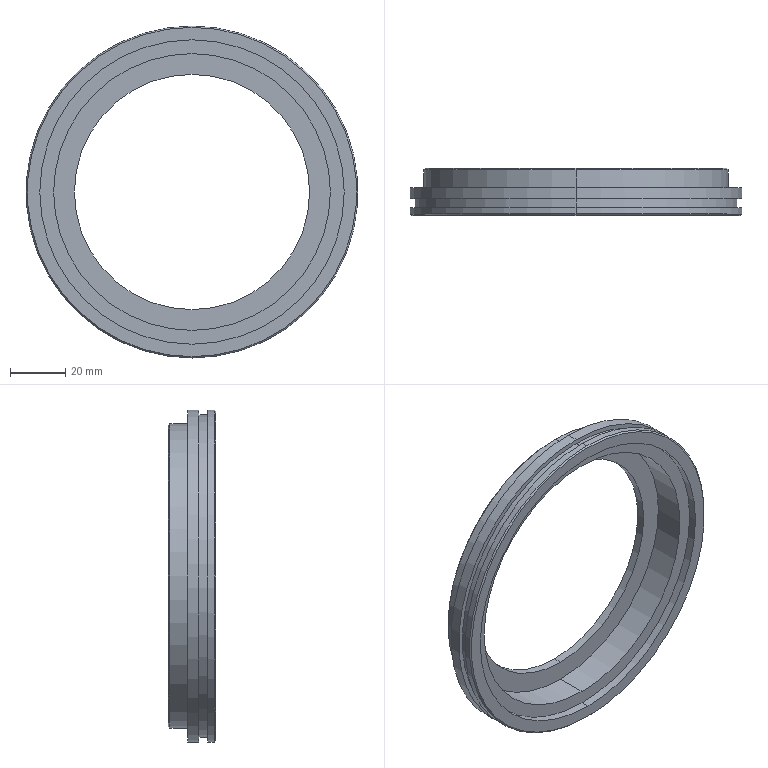Part | SolidWorks | features ICE 5, Chamfer 2, Extrusion 1 | 1 solid | 25 faces | box 120 x 17 x 120 mm | volume 45523 mm3 | cylinder 14 | plane 7 | cone 4 | commonest cylinder face diameters 110 x4 120 x4 85 x2 100 x2 116.5 x2
STEP:
#1=CARTESIAN_POINT('',(0.,17.,54.5));
#2=VERTEX_POINT('',#1);
#3=CARTESIAN_POINT('',(0.,17.,-54.5));
#4=VERTEX_POINT('',#3);
#5=CARTESIAN_POINT('',(0.,17.,0.));
#6=DIRECTION('',(0.,1.,0.));
#7=DIRECTION('',(0.,0.,1.));
#8=AXIS2_PLACEMENT_3D('',#5,#6,#7);
#9=CIRCLE('',#8,54.5);
#10=EDGE_CURVE('',#2,#4,#9,.T.);
#11=ORIENTED_EDGE('',*,*,#10,.F.);
#12=CARTESIAN_POINT('',(0.,16.5,55.));
#13=VERTEX_POINT('',#12);
#14=CARTESIAN_POINT('',(0.,17.,54.5));
#15=DIRECTION('',(0.,-0.7071,0.7071));
#16=VECTOR('',#15,1000.);
#17=LINE('',#14,#16);
#18=EDGE_CURVE('',#2,#13,#17,.T.);
#19=ORIENTED_EDGE('',*,*,#18,.T.);
#20=CARTESIAN_POINT('',(0.,16.5,-55.));
#21=VERTEX_POINT('',#20);
#22=CARTESIAN_POINT('',(0.,16.5,0.));
#23=DIRECTION('',(0.,-1.,0.));
#24=DIRECTION('',(0.,0.,1.));
#25=AXIS2_PLACEMENT_3D('',#22,#23,#24);
#26=CIRCLE('',#25,55.);
#27=EDGE_CURVE('',#21,#13,#26,.T.);
#28=ORIENTED_EDGE('',*,*,#27,.F.);
#29=CARTESIAN_POINT('',(0.,17.,-54.5));
#30=DIRECTION('',(0.,-0.7071,-0.7071));
#31=VECTOR('',#30,1000.);
#32=LINE('',#29,#31);
#33=EDGE_CURVE('',#4,#21,#32,.T.);
#34=ORIENTED_EDGE('',*,*,#33,.F.);
#35=EDGE_LOOP('',(#11,#19,#28,#34));
#36=FACE_OUTER_BOUND('',#35,.T.);
#37=CARTESIAN_POINT('',(0.,17.,0.));
#38=DIRECTION('',(0.,-1.,0.));
#39=DIRECTION('',(0.,0.,-1.));
#40=AXIS2_PLACEMENT_3D('',#37,#38,#39);
#41=CONICAL_SURFACE('',#40,54.5,0.7854);
#42=ADVANCED_FACE('',(#36),#41,.T.);
#43=CARTESIAN_POINT('',(0.,0.,-59.5));
#44=VERTEX_POINT('',#43);
#45=CARTESIAN_POINT('',(0.,0.,59.5));
#46=VERTEX_POINT('',#45);
#47=CARTESIAN_POINT('',(0.,0.,0.));
#48=DIRECTION('',(0.,-1.,0.));
#49=DIRECTION('',(0.,0.,1.));
#50=AXIS2_PLACEMENT_3D('',#47,#48,#49);
#51=CIRCLE('',#50,59.5);
#52=EDGE_CURVE('',#44,#46,#51,.T.);
#53=ORIENTED_EDGE('',*,*,#52,.F.);
#54=CARTESIAN_POINT('',(0.,0.5,-60.));
#55=VERTEX_POINT('',#54);
#56=CARTESIAN_POINT('',(0.,0.5,-60.));
#57=DIRECTION('',(0.,0.7071,-0.7071));
#58=VECTOR('',#57,1000.);
#59=LINE('',#56,#58);
#60=EDGE_CURVE('',#44,#55,#59,.T.);
#61=ORIENTED_EDGE('',*,*,#60,.T.);
#62=CARTESIAN_POINT('',(0.,0.5,60.));
#63=VERTEX_POINT('',#62);
#64=CARTESIAN_POINT('',(0.,0.5,0.));
#65=DIRECTION('',(0.,1.,0.));
#66=DIRECTION('',(0.,0.,1.));
#67=AXIS2_PLACEMENT_3D('',#64,#65,#66);
#68=CIRCLE('',#67,60.);
#69=EDGE_CURVE('',#63,#55,#68,.T.);
#70=ORIENTED_EDGE('',*,*,#69,.F.);
#71=CARTESIAN_POINT('',(0.,0.5,60.));
#72=DIRECTION('',(0.,0.7071,0.7071));
#73=VECTOR('',#72,1000.);
#74=LINE('',#71,#73);
#75=EDGE_CURVE('',#46,#63,#74,.T.);
#76=ORIENTED_EDGE('',*,*,#75,.F.);
#77=EDGE_LOOP('',(#53,#61,#70,#76));
#78=FACE_OUTER_BOUND('',#77,.T.);
#79=CARTESIAN_POINT('',(0.,0.5,0.));
#80=DIRECTION('',(0.,1.,0.));
#81=DIRECTION('',(0.,0.,1.));
#82=AXIS2_PLACEMENT_3D('',#79,#80,#81);
#83=CONICAL_SURFACE('',#82,60.,0.7854);
#84=ADVANCED_FACE('',(#78),#83,.T.);
#85=CARTESIAN_POINT('',(0.,2.8,-58.25));
#86=VERTEX_POINT('',#85);
#87=CARTESIAN_POINT('',(0.,2.8,58.25));
#88=VERTEX_POINT('',#87);
#89=CARTESIAN_POINT('',(0.,2.8,0.));
#90=DIRECTION('',(0.,-1.,0.));
#91=DIRECTION('',(0.,0.,-1.));
#92=AXIS2_PLACEMENT_3D('',#89,#90,#91);
#93=CIRCLE('',#92,58.25);
#94=EDGE_CURVE('',#86,#88,#93,.T.);
#95=ORIENTED_EDGE('',*,*,#94,.F.);
#96=CARTESIAN_POINT('',(0.,6.,-58.25));
#97=VERTEX_POINT('',#96);
#98=CARTESIAN_POINT('',(0.,2.8,-58.25));
#99=DIRECTION('',(0.,1.,0.));
#100=VECTOR('',#99,1000.);
#101=LINE('',#98,#100);
#102=EDGE_CURVE('',#86,#97,#101,.T.);
#103=ORIENTED_EDGE('',*,*,#102,.T.);
#104=CARTESIAN_POINT('',(0.,6.,58.25));
#105=VERTEX_POINT('',#104);
#106=CARTESIAN_POINT('',(0.,6.,0.));
#107=DIRECTION('',(0.,-1.,0.));
#108=DIRECTION('',(0.,0.,-1.));
#109=AXIS2_PLACEMENT_3D('',#106,#107,#108);
#110=CIRCLE('',#109,58.25);
#111=EDGE_CURVE('',#97,#105,#110,.T.);
#112=ORIENTED_EDGE('',*,*,#111,.T.);
#113=CARTESIAN_POINT('',(0.,2.8,58.25));
#114=DIRECTION('',(0.,1.,0.));
#115=VECTOR('',#114,1000.);
#116=LINE('',#113,#115);
#117=EDGE_CURVE('',#88,#105,#116,.T.);
#118=ORIENTED_EDGE('',*,*,#117,.F.);
#119=EDGE_LOOP('',(#95,#103,#112,#118));
#120=FACE_OUTER_BOUND('',#119,.T.);
#121=CARTESIAN_POINT('',(0.,2.8,0.));
#122=DIRECTION('',(0.,1.,0.));
#123=DIRECTION('',(0.,0.,1.));
#124=AXIS2_PLACEMENT_3D('',#121,#122,#123);
#125=CYLINDRICAL_SURFACE('',#124,58.25);
#126=ADVANCED_FACE('',(#120),#125,.T.);
#127=CARTESIAN_POINT('',(0.,14.,50.));
#128=VERTEX_POINT('',#127);
#129=CARTESIAN_POINT('',(0.,14.,-50.));
#130=VERTEX_POINT('',#129);
#131=CARTESIAN_POINT('',(0.,14.,0.));
#132=DIRECTION('',(0.,-1.,0.));
#133=DIRECTION('',(0.,0.,-1.));
#134=AXIS2_PLACEMENT_3D('',#131,#132,#133);
#135=CIRCLE('',#134,50.);
#136=EDGE_CURVE('',#128,#130,#135,.T.);
#137=ORIENTED_EDGE('',*,*,#136,.F.);
#138=CARTESIAN_POINT('',(0.,3.,50.));
#139=VERTEX_POINT('',#138);
#140=CARTESIAN_POINT('',(0.,14.,50.));
#141=DIRECTION('',(0.,-1.,0.));
#142=VECTOR('',#141,1000.);
#143=LINE('',#140,#142);
#144=EDGE_CURVE('',#128,#139,#143,.T.);
#145=ORIENTED_EDGE('',*,*,#144,.T.);
#146=CARTESIAN_POINT('',(0.,3.,-50.));
#147=VERTEX_POINT('',#146);
#148=CARTESIAN_POINT('',(0.,3.,0.));
#149=DIRECTION('',(0.,-1.,0.));
#150=DIRECTION('',(0.,0.,-1.));
#151=AXIS2_PLACEMENT_3D('',#148,#149,#150);
#152=CIRCLE('',#151,50.);
#153=EDGE_CURVE('',#139,#147,#152,.T.);
#154=ORIENTED_EDGE('',*,*,#153,.T.);
#155=CARTESIAN_POINT('',(0.,14.,-50.));
#156=DIRECTION('',(0.,-1.,0.));
#157=VECTOR('',#156,1000.);
#158=LINE('',#155,#157);
#159=EDGE_CURVE('',#130,#147,#158,.T.);
#160=ORIENTED_EDGE('',*,*,#159,.F.);
#161=EDGE_LOOP('',(#137,#145,#154,#160));
#162=FACE_OUTER_BOUND('',#161,.T.);
#163=CARTESIAN_POINT('',(0.,14.,0.));
#164=DIRECTION('',(0.,-1.,0.));
#165=DIRECTION('',(0.,0.,-1.));
#166=AXIS2_PLACEMENT_3D('',#163,#164,#165);
#167=CYLINDRICAL_SURFACE('',#166,50.);
#168=ADVANCED_FACE('',(#162),#167,.F.);
#169=CARTESIAN_POINT('',(0.,3.,55.));
#170=VERTEX_POINT('',#169);
#171=CARTESIAN_POINT('',(0.,3.,-55.));
#172=VERTEX_POINT('',#171);
#173=CARTESIAN_POINT('',(0.,3.,0.));
#174=DIRECTION('',(0.,-1.,0.));
#175=DIRECTION('',(0.,0.,-1.));
#176=AXIS2_PLACEMENT_3D('',#173,#174,#175);
#177=CIRCLE('',#176,55.);
#178=EDGE_CURVE('',#170,#172,#177,.T.);
#179=ORIENTED_EDGE('',*,*,#178,.F.);
#180=CARTESIAN_POINT('',(0.,0.,55.));
#181=VERTEX_POINT('',#180);
#182=CARTESIAN_POINT('',(0.,3.,55.));
#183=DIRECTION('',(0.,-1.,0.));
#184=VECTOR('',#183,1000.);
#185=LINE('',#182,#184);
#186=EDGE_CURVE('',#170,#181,#185,.T.);
#187=ORIENTED_EDGE('',*,*,#186,.T.);
#188=CARTESIAN_POINT('',(0.,0.,-55.));
#189=VERTEX_POINT('',#188);
#190=CARTESIAN_POINT('',(0.,0.,0.));
#191=DIRECTION('',(0.,-1.,0.));
#192=DIRECTION('',(0.,0.,-1.));
#193=AXIS2_PLACEMENT_3D('',#190,#191,#192);
#194=CIRCLE('',#193,55.);
#195=EDGE_CURVE('',#181,#189,#194,.T.);
#196=ORIENTED_EDGE('',*,*,#195,.T.);
#197=CARTESIAN_POINT('',(0.,3.,-55.));
#198=DIRECTION('',(0.,-1.,0.));
#199=VECTOR('',#198,1000.);
#200=LINE('',#197,#199);
#201=EDGE_CURVE('',#172,#189,#200,.T.);
#202=ORIENTED_EDGE('',*,*,#201,.F.);
#203=EDGE_LOOP('',(#179,#187,#196,#202));
#204=FACE_OUTER_BOUND('',#203,.T.);
#205=CARTESIAN_POINT('',(0.,3.,0.));
#206=DIRECTION('',(0.,-1.,0.));
#207=DIRECTION('',(0.,0.,-1.));
#208=AXIS2_PLACEMENT_3D('',#205,#206,#207);
#209=CYLINDRICAL_SURFACE('',#208,55.);
#210=ADVANCED_FACE('',(#204),#209,.F.);
#211=ORIENTED_EDGE('',*,*,#27,.T.);
#212=CARTESIAN_POINT('',(0.,10.,55.));
#213=VERTEX_POINT('',#212);
#214=CARTESIAN_POINT('',(0.,17.,55.));
#215=DIRECTION('',(0.,-1.,0.));
#216=VECTOR('',#215,1000.);
#217=LINE('',#214,#216);
#218=EDGE_CURVE('',#13,#213,#217,.T.);
#219=ORIENTED_EDGE('',*,*,#218,.T.);
#220=CARTESIAN_POINT('',(0.,10.,-55.));
#221=VERTEX_POINT('',#220);
#222=CARTESIAN_POINT('',(0.,10.,0.));
#223=DIRECTION('',(0.,1.,0.));
#224=DIRECTION('',(0.,0.,1.));
#225=AXIS2_PLACEMENT_3D('',#222,#223,#224);
#226=CIRCLE('',#225,55.);
#227=EDGE_CURVE('',#213,#221,#226,.T.);
#228=ORIENTED_EDGE('',*,*,#227,.T.);
#229=CARTESIAN_POINT('',(0.,17.,-55.));
#230=DIRECTION('',(0.,-1.,0.));
#231=VECTOR('',#230,1000.);
#232=LINE('',#229,#231);
#233=EDGE_CURVE('',#21,#221,#232,.T.);
#234=ORIENTED_EDGE('',*,*,#233,.F.);
#235=EDGE_LOOP('',(#211,#219,#228,#234));
#236=FACE_OUTER_BOUND('',#235,.T.);
#237=CARTESIAN_POINT('',(0.,17.,0.));
#238=DIRECTION('',(0.,-1.,0.));
#239=DIRECTION('',(0.,0.,-1.));
#240=AXIS2_PLACEMENT_3D('',#237,#238,#239);
#241=CYLINDRICAL_SURFACE('',#240,55.);
#242=ADVANCED_FACE('',(#236),#241,.T.);
#243=CARTESIAN_POINT('',(0.,2.8,-60.));
#244=VERTEX_POINT('',#243);
#245=CARTESIAN_POINT('',(0.,2.8,60.));
#246=VERTEX_POINT('',#245);
#247=CARTESIAN_POINT('',(0.,2.8,0.));
#248=DIRECTION('',(0.,-1.,0.));
#249=DIRECTION('',(0.,0.,-1.));
#250=AXIS2_PLACEMENT_3D('',#247,#248,#249);
#251=CIRCLE('',#250,60.);
#252=EDGE_CURVE('',#244,#246,#251,.T.);
#253=ORIENTED_EDGE('',*,*,#252,.T.);
#254=CARTESIAN_POINT('',(0.,10.,60.));
#255=DIRECTION('',(0.,-1.,0.));
#256=VECTOR('',#255,1000.);
#257=LINE('',#254,#256);
#258=EDGE_CURVE('',#246,#63,#257,.T.);
#259=ORIENTED_EDGE('',*,*,#258,.T.);
#260=ORIENTED_EDGE('',*,*,#69,.T.);
#261=CARTESIAN_POINT('',(0.,10.,-60.));
#262=DIRECTION('',(0.,-1.,0.));
#263=VECTOR('',#262,1000.);
#264=LINE('',#261,#263);
#265=EDGE_CURVE('',#244,#55,#264,.T.);
#266=ORIENTED_EDGE('',*,*,#265,.F.);
#267=EDGE_LOOP('',(#253,#259,#260,#266));
#268=FACE_OUTER_BOUND('',#267,.T.);
#269=CARTESIAN_POINT('',(0.,10.,0.));
#270=DIRECTION('',(0.,-1.,0.));
#271=DIRECTION('',(0.,0.,-1.));
#272=AXIS2_PLACEMENT_3D('',#269,#270,#271);
#273=CYLINDRICAL_SURFACE('',#272,60.);
#274=ADVANCED_FACE('',(#268),#273,.T.);
#275=CARTESIAN_POINT('',(0.,14.,-42.5));
#276=VERTEX_POINT('',#275);
#277=CARTESIAN_POINT('',(0.,14.,42.5));
#278=VERTEX_POINT('',#277);
#279=CARTESIAN_POINT('',(0.,14.,0.));
#280=DIRECTION('',(0.,1.,0.));
#281=DIRECTION('',(0.,0.,-1.));
#282=AXIS2_PLACEMENT_3D('',#279,#280,#281);
#283=CIRCLE('',#282,42.5);
#284=EDGE_CURVE('',#276,#278,#283,.T.);
#285=ORIENTED_EDGE('',*,*,#284,.F.);
#286=CARTESIAN_POINT('',(0.,17.,-42.5));
#287=VERTEX_POINT('',#286);
#288=CARTESIAN_POINT('',(0.,0.,-42.5));
#289=DIRECTION('',(0.,1.,0.));
#290=VECTOR('',#289,1000.);
#291=LINE('',#288,#290);
#292=EDGE_CURVE('',#276,#287,#291,.T.);
#293=ORIENTED_EDGE('',*,*,#292,.T.);
#294=CARTESIAN_POINT('',(0.,17.,42.5));
#295=VERTEX_POINT('',#294);
#296=CARTESIAN_POINT('',(0.,17.,0.));
#297=DIRECTION('',(0.,1.,0.));
#298=DIRECTION('',(0.,0.,1.));
#299=AXIS2_PLACEMENT_3D('',#296,#297,#298);
#300=CIRCLE('',#299,42.5);
#301=EDGE_CURVE('',#287,#295,#300,.T.);
#302=ORIENTED_EDGE('',*,*,#301,.T.);
#303=CARTESIAN_POINT('',(0.,0.,42.5));
#304=DIRECTION('',(0.,1.,0.));
#305=VECTOR('',#304,1000.);
#306=LINE('',#303,#305);
#307=EDGE_CURVE('',#278,#295,#306,.T.);
#308=ORIENTED_EDGE('',*,*,#307,.F.);
#309=EDGE_LOOP('',(#285,#293,#302,#308));
#310=FACE_OUTER_BOUND('',#309,.T.);
#311=CARTESIAN_POINT('',(0.,0.,0.));
#312=DIRECTION('',(0.,1.,0.));
#313=DIRECTION('',(0.,0.,1.));
#314=AXIS2_PLACEMENT_3D('',#311,#312,#313);
#315=CYLINDRICAL_SURFACE('',#314,42.5);
#316=ADVANCED_FACE('',(#310),#315,.F.);
#317=CARTESIAN_POINT('',(0.,10.,60.));
#318=VERTEX_POINT('',#317);
#319=CARTESIAN_POINT('',(0.,10.,-60.));
#320=VERTEX_POINT('',#319);
#321=CARTESIAN_POINT('',(0.,10.,0.));
#322=DIRECTION('',(0.,1.,0.));
#323=DIRECTION('',(0.,0.,1.));
#324=AXIS2_PLACEMENT_3D('',#321,#322,#323);
#325=CIRCLE('',#324,60.);
#326=EDGE_CURVE('',#318,#320,#325,.T.);
#327=ORIENTED_EDGE('',*,*,#326,.F.);
#328=CARTESIAN_POINT('',(0.,6.,60.));
#329=VERTEX_POINT('',#328);
#330=CARTESIAN_POINT('',(0.,10.,60.));
#331=DIRECTION('',(0.,-1.,0.));
#332=VECTOR('',#331,1000.);
#333=LINE('',#330,#332);
#334=EDGE_CURVE('',#318,#329,#333,.T.);
#335=ORIENTED_EDGE('',*,*,#334,.T.);
#336=CARTESIAN_POINT('',(0.,6.,-60.));
#337=VERTEX_POINT('',#336);
#338=CARTESIAN_POINT('',(0.,6.,0.));
#339=DIRECTION('',(0.,-1.,0.));
#340=DIRECTION('',(0.,0.,-1.));
#341=AXIS2_PLACEMENT_3D('',#338,#339,#340);
#342=CIRCLE('',#341,60.);
#343=EDGE_CURVE('',#337,#329,#342,.T.);
#344=ORIENTED_EDGE('',*,*,#343,.F.);
#345=CARTESIAN_POINT('',(0.,10.,-60.));
#346=DIRECTION('',(0.,-1.,0.));
#347=VECTOR('',#346,1000.);
#348=LINE('',#345,#347);
#349=EDGE_CURVE('',#320,#337,#348,.T.);
#350=ORIENTED_EDGE('',*,*,#349,.F.);
#351=EDGE_LOOP('',(#327,#335,#344,#350));
#352=FACE_OUTER_BOUND('',#351,.T.);
#353=CARTESIAN_POINT('',(0.,10.,0.));
#354=DIRECTION('',(0.,-1.,0.));
#355=DIRECTION('',(0.,0.,-1.));
#356=AXIS2_PLACEMENT_3D('',#353,#354,#355);
#357=CYLINDRICAL_SURFACE('',#356,60.);
#358=ADVANCED_FACE('',(#352),#357,.T.);
#359=ORIENTED_EDGE('',*,*,#334,.F.);
#360=CARTESIAN_POINT('',(0.,10.,0.));
#361=DIRECTION('',(0.,1.,0.));
#362=DIRECTION('',(0.,0.,1.));
#363=AXIS2_PLACEMENT_3D('',#360,#361,#362);
#364=CIRCLE('',#363,60.);
#365=EDGE_CURVE('',#320,#318,#364,.T.);
#366=ORIENTED_EDGE('',*,*,#365,.F.);
#367=ORIENTED_EDGE('',*,*,#349,.T.);
#368=CARTESIAN_POINT('',(0.,6.,0.));
#369=DIRECTION('',(0.,-1.,0.));
#370=DIRECTION('',(0.,0.,-1.));
#371=AXIS2_PLACEMENT_3D('',#368,#369,#370);
#372=CIRCLE('',#371,60.);
#373=EDGE_CURVE('',#329,#337,#372,.T.);
#374=ORIENTED_EDGE('',*,*,#373,.F.);
#375=EDGE_LOOP('',(#359,#366,#367,#374));
#376=FACE_OUTER_BOUND('',#375,.T.);
#377=CARTESIAN_POINT('',(0.,10.,0.));
#378=DIRECTION('',(0.,-1.,0.));
#379=DIRECTION('',(0.,0.,-1.));
#380=AXIS2_PLACEMENT_3D('',#377,#378,#379);
#381=CYLINDRICAL_SURFACE('',#380,60.);
#382=ADVANCED_FACE('',(#376),#381,.T.);
#383=ORIENTED_EDGE('',*,*,#292,.F.);
#384=CARTESIAN_POINT('',(0.,14.,0.));
#385=DIRECTION('',(0.,1.,0.));
#386=DIRECTION('',(0.,0.,-1.));
#387=AXIS2_PLACEMENT_3D('',#384,#385,#386);
#388=CIRCLE('',#387,42.5);
#389=EDGE_CURVE('',#278,#276,#388,.T.);
#390=ORIENTED_EDGE('',*,*,#389,.F.);
#391=ORIENTED_EDGE('',*,*,#307,.T.);
#392=CARTESIAN_POINT('',(0.,17.,0.));
#393=DIRECTION('',(0.,1.,0.));
#394=DIRECTION('',(0.,0.,1.));
#395=AXIS2_PLACEMENT_3D('',#392,#393,#394);
#396=CIRCLE('',#395,42.5);
#397=EDGE_CURVE('',#295,#287,#396,.T.);
#398=ORIENTED_EDGE('',*,*,#397,.T.);
#399=EDGE_LOOP('',(#383,#390,#391,#398));
#400=FACE_OUTER_BOUND('',#399,.T.);
#401=CARTESIAN_POINT('',(0.,0.,0.));
#402=DIRECTION('',(0.,1.,0.));
#403=DIRECTION('',(0.,0.,1.));
#404=AXIS2_PLACEMENT_3D('',#401,#402,#403);
#405=CYLINDRICAL_SURFACE('',#404,42.5);
#406=ADVANCED_FACE('',(#400),#405,.F.);
#407=ORIENTED_EDGE('',*,*,#258,.F.);
#408=CARTESIAN_POINT('',(0.,2.8,0.));
#409=DIRECTION('',(0.,-1.,0.));
#410=DIRECTION('',(0.,0.,-1.));
#411=AXIS2_PLACEMENT_3D('',#408,#409,#410);
#412=CIRCLE('',#411,60.);
#413=EDGE_CURVE('',#246,#244,#412,.T.);
#414=ORIENTED_EDGE('',*,*,#413,.T.);
#415=ORIENTED_EDGE('',*,*,#265,.T.);
#416=CARTESIAN_POINT('',(0.,0.5,0.));
#417=DIRECTION('',(0.,1.,0.));
#418=DIRECTION('',(0.,0.,1.));
#419=AXIS2_PLACEMENT_3D('',#416,#417,#418);
#420=CIRCLE('',#419,60.);
#421=EDGE_CURVE('',#55,#63,#420,.T.);
#422=ORIENTED_EDGE('',*,*,#421,.T.);
#423=EDGE_LOOP('',(#407,#414,#415,#422));
#424=FACE_OUTER_BOUND('',#423,.T.);
#425=CARTESIAN_POINT('',(0.,10.,0.));
#426=DIRECTION('',(0.,-1.,0.));
#427=DIRECTION('',(0.,0.,-1.));
#428=AXIS2_PLACEMENT_3D('',#425,#426,#427);
#429=CYLINDRICAL_SURFACE('',#428,60.);
#430=ADVANCED_FACE('',(#424),#429,.T.);
#431=CARTESIAN_POINT('',(0.,10.,0.));
#432=DIRECTION('',(0.,1.,0.));
#433=DIRECTION('',(0.,0.,1.));
#434=AXIS2_PLACEMENT_3D('',#431,#432,#433);
#435=CIRCLE('',#434,55.);
#436=EDGE_CURVE('',#221,#213,#435,.T.);
#437=ORIENTED_EDGE('',*,*,#436,.F.);
#438=ORIENTED_EDGE('',*,*,#227,.F.);
#439=EDGE_LOOP('',(#437,#438));
#440=FACE_BOUND('',#439,.T.);
#441=ORIENTED_EDGE('',*,*,#365,.T.);
#442=ORIENTED_EDGE('',*,*,#326,.T.);
#443=EDGE_LOOP('',(#441,#442));
#444=FACE_OUTER_BOUND('',#443,.T.);
#445=CARTESIAN_POINT('',(0.,10.,0.));
#446=DIRECTION('',(0.,1.,0.));
#447=DIRECTION('',(0.,0.,1.));
#448=AXIS2_PLACEMENT_3D('',#445,#446,#447);
#449=PLANE('',#448);
#450=ADVANCED_FACE('',(#440,#444),#449,.T.);
#451=CARTESIAN_POINT('',(0.,0.,0.));
#452=DIRECTION('',(0.,-1.,0.));
#453=DIRECTION('',(0.,0.,1.));
#454=AXIS2_PLACEMENT_3D('',#451,#452,#453);
#455=CIRCLE('',#454,59.5);
#456=EDGE_CURVE('',#46,#44,#455,.T.);
#457=ORIENTED_EDGE('',*,*,#456,.T.);
#458=ORIENTED_EDGE('',*,*,#52,.T.);
#459=EDGE_LOOP('',(#457,#458));
#460=FACE_OUTER_BOUND('',#459,.T.);
#461=CARTESIAN_POINT('',(0.,0.,0.));
#462=DIRECTION('',(0.,-1.,0.));
#463=DIRECTION('',(0.,0.,-1.));
#464=AXIS2_PLACEMENT_3D('',#461,#462,#463);
#465=CIRCLE('',#464,55.);
#466=EDGE_CURVE('',#189,#181,#465,.T.);
#467=ORIENTED_EDGE('',*,*,#466,.F.);
#468=ORIENTED_EDGE('',*,*,#195,.F.);
#469=EDGE_LOOP('',(#467,#468));
#470=FACE_BOUND('',#469,.T.);
#471=CARTESIAN_POINT('',(0.,0.,0.));
#472=DIRECTION('',(0.,1.,0.));
#473=DIRECTION('',(0.,0.,1.));
#474=AXIS2_PLACEMENT_3D('',#471,#472,#473);
#475=PLANE('',#474);
#476=ADVANCED_FACE('',(#460,#470),#475,.F.);
#477=ORIENTED_EDGE('',*,*,#218,.F.);
#478=CARTESIAN_POINT('',(0.,16.5,0.));
#479=DIRECTION('',(0.,-1.,0.));
#480=DIRECTION('',(0.,0.,1.));
#481=AXIS2_PLACEMENT_3D('',#478,#479,#480);
#482=CIRCLE('',#481,55.);
#483=EDGE_CURVE('',#13,#21,#482,.T.);
#484=ORIENTED_EDGE('',*,*,#483,.T.);
#485=ORIENTED_EDGE('',*,*,#233,.T.);
#486=ORIENTED_EDGE('',*,*,#436,.T.);
#487=EDGE_LOOP('',(#477,#484,#485,#486));
#488=FACE_OUTER_BOUND('',#487,.T.);
#489=CARTESIAN_POINT('',(0.,17.,0.));
#490=DIRECTION('',(0.,-1.,0.));
#491=DIRECTION('',(0.,0.,-1.));
#492=AXIS2_PLACEMENT_3D('',#489,#490,#491);
#493=CYLINDRICAL_SURFACE('',#492,55.);
#494=ADVANCED_FACE('',(#488),#493,.T.);
#495=CARTESIAN_POINT('',(0.,17.,0.));
#496=DIRECTION('',(0.,1.,0.));
#497=DIRECTION('',(0.,0.,1.));
#498=AXIS2_PLACEMENT_3D('',#495,#496,#497);
#499=CIRCLE('',#498,54.5);
#500=EDGE_CURVE('',#4,#2,#499,.T.);
#501=ORIENTED_EDGE('',*,*,#500,.T.);
#502=ORIENTED_EDGE('',*,*,#10,.T.);
#503=EDGE_LOOP('',(#501,#502));
#504=FACE_OUTER_BOUND('',#503,.T.);
#505=ORIENTED_EDGE('',*,*,#397,.F.);
#506=ORIENTED_EDGE('',*,*,#301,.F.);
#507=EDGE_LOOP('',(#505,#506));
#508=FACE_BOUND('',#507,.T.);
#509=CARTESIAN_POINT('',(0.,17.,0.));
#510=DIRECTION('',(0.,1.,0.));
#511=DIRECTION('',(0.,0.,1.));
#512=AXIS2_PLACEMENT_3D('',#509,#510,#511);
#513=PLANE('',#512);
#514=ADVANCED_FACE('',(#504,#508),#513,.T.);
#515=CARTESIAN_POINT('',(0.,3.,0.));
#516=DIRECTION('',(0.,-1.,0.));
#517=DIRECTION('',(0.,0.,-1.));
#518=AXIS2_PLACEMENT_3D('',#515,#516,#517);
#519=CIRCLE('',#518,50.);
#520=EDGE_CURVE('',#147,#139,#519,.T.);
#521=ORIENTED_EDGE('',*,*,#520,.F.);
#522=ORIENTED_EDGE('',*,*,#153,.F.);
#523=EDGE_LOOP('',(#521,#522));
#524=FACE_BOUND('',#523,.T.);
#525=CARTESIAN_POINT('',(0.,3.,0.));
#526=DIRECTION('',(0.,-1.,0.));
#527=DIRECTION('',(0.,0.,-1.));
#528=AXIS2_PLACEMENT_3D('',#525,#526,#527);
#529=CIRCLE('',#528,55.);
#530=EDGE_CURVE('',#172,#170,#529,.T.);
#531=ORIENTED_EDGE('',*,*,#530,.T.);
#532=ORIENTED_EDGE('',*,*,#178,.T.);
#533=EDGE_LOOP('',(#531,#532));
#534=FACE_OUTER_BOUND('',#533,.T.);
#535=CARTESIAN_POINT('',(0.,3.,0.));
#536=DIRECTION('',(0.,-1.,0.));
#537=DIRECTION('',(0.,0.,-1.));
#538=AXIS2_PLACEMENT_3D('',#535,#536,#537);
#539=PLANE('',#538);
#540=ADVANCED_FACE('',(#524,#534),#539,.T.);
#541=ORIENTED_EDGE('',*,*,#186,.F.);
#542=ORIENTED_EDGE('',*,*,#530,.F.);
#543=ORIENTED_EDGE('',*,*,#201,.T.);
#544=ORIENTED_EDGE('',*,*,#466,.T.);
#545=EDGE_LOOP('',(#541,#542,#543,#544));
#546=FACE_OUTER_BOUND('',#545,.T.);
#547=CARTESIAN_POINT('',(0.,3.,0.));
#548=DIRECTION('',(0.,-1.,0.));
#549=DIRECTION('',(0.,0.,-1.));
#550=AXIS2_PLACEMENT_3D('',#547,#548,#549);
#551=CYLINDRICAL_SURFACE('',#550,55.);
#552=ADVANCED_FACE('',(#546),#551,.F.);
#553=CARTESIAN_POINT('',(0.,14.,0.));
#554=DIRECTION('',(0.,-1.,0.));
#555=DIRECTION('',(0.,0.,-1.));
#556=AXIS2_PLACEMENT_3D('',#553,#554,#555);
#557=CIRCLE('',#556,50.);
#558=EDGE_CURVE('',#130,#128,#557,.T.);
#559=ORIENTED_EDGE('',*,*,#558,.T.);
#560=ORIENTED_EDGE('',*,*,#136,.T.);
#561=EDGE_LOOP('',(#559,#560));
#562=FACE_OUTER_BOUND('',#561,.T.);
#563=ORIENTED_EDGE('',*,*,#389,.T.);
#564=ORIENTED_EDGE('',*,*,#284,.T.);
#565=EDGE_LOOP('',(#563,#564));
#566=FACE_BOUND('',#565,.T.);
#567=CARTESIAN_POINT('',(0.,14.,0.));
#568=DIRECTION('',(0.,-1.,0.));
#569=DIRECTION('',(0.,0.,-1.));
#570=AXIS2_PLACEMENT_3D('',#567,#568,#569);
#571=PLANE('',#570);
#572=ADVANCED_FACE('',(#562,#566),#571,.T.);
#573=ORIENTED_EDGE('',*,*,#144,.F.);
#574=ORIENTED_EDGE('',*,*,#558,.F.);
#575=ORIENTED_EDGE('',*,*,#159,.T.);
#576=ORIENTED_EDGE('',*,*,#520,.T.);
#577=EDGE_LOOP('',(#573,#574,#575,#576));
#578=FACE_OUTER_BOUND('',#577,.T.);
#579=CARTESIAN_POINT('',(0.,14.,0.));
#580=DIRECTION('',(0.,-1.,0.));
#581=DIRECTION('',(0.,0.,-1.));
#582=AXIS2_PLACEMENT_3D('',#579,#580,#581);
#583=CYLINDRICAL_SURFACE('',#582,50.);
#584=ADVANCED_FACE('',(#578),#583,.F.);
#585=CARTESIAN_POINT('',(0.,2.8,0.));
#586=DIRECTION('',(0.,-1.,0.));
#587=DIRECTION('',(0.,0.,-1.));
#588=AXIS2_PLACEMENT_3D('',#585,#586,#587);
#589=CIRCLE('',#588,58.25);
#590=EDGE_CURVE('',#88,#86,#589,.T.);
#591=ORIENTED_EDGE('',*,*,#590,.T.);
#592=ORIENTED_EDGE('',*,*,#94,.T.);
#593=EDGE_LOOP('',(#591,#592));
#594=FACE_BOUND('',#593,.T.);
#595=ORIENTED_EDGE('',*,*,#252,.F.);
#596=ORIENTED_EDGE('',*,*,#413,.F.);
#597=EDGE_LOOP('',(#595,#596));
#598=FACE_OUTER_BOUND('',#597,.T.);
#599=CARTESIAN_POINT('',(0.,2.8,0.));
#600=DIRECTION('',(0.,-1.,0.));
#601=DIRECTION('',(0.,0.,-1.));
#602=AXIS2_PLACEMENT_3D('',#599,#600,#601);
#603=PLANE('',#602);
#604=ADVANCED_FACE('',(#594,#598),#603,.F.);
#605=CARTESIAN_POINT('',(0.,6.,0.));
#606=DIRECTION('',(0.,-1.,0.));
#607=DIRECTION('',(0.,0.,-1.));
#608=AXIS2_PLACEMENT_3D('',#605,#606,#607);
#609=CIRCLE('',#608,58.25);
#610=EDGE_CURVE('',#105,#97,#609,.T.);
#611=ORIENTED_EDGE('',*,*,#610,.F.);
#612=ORIENTED_EDGE('',*,*,#111,.F.);
#613=EDGE_LOOP('',(#611,#612));
#614=FACE_BOUND('',#613,.T.);
#615=ORIENTED_EDGE('',*,*,#343,.T.);
#616=ORIENTED_EDGE('',*,*,#373,.T.);
#617=EDGE_LOOP('',(#615,#616));
#618=FACE_OUTER_BOUND('',#617,.T.);
#619=CARTESIAN_POINT('',(0.,6.,0.));
#620=DIRECTION('',(0.,-1.,0.));
#621=DIRECTION('',(0.,0.,-1.));
#622=AXIS2_PLACEMENT_3D('',#619,#620,#621);
#623=PLANE('',#622);
#624=ADVANCED_FACE('',(#614,#618),#623,.T.);
#625=ORIENTED_EDGE('',*,*,#102,.F.);
#626=ORIENTED_EDGE('',*,*,#590,.F.);
#627=ORIENTED_EDGE('',*,*,#117,.T.);
#628=ORIENTED_EDGE('',*,*,#610,.T.);
#629=EDGE_LOOP('',(#625,#626,#627,#628));
#630=FACE_OUTER_BOUND('',#629,.T.);
#631=CARTESIAN_POINT('',(0.,2.8,0.));
#632=DIRECTION('',(0.,1.,0.));
#633=DIRECTION('',(0.,0.,1.));
#634=AXIS2_PLACEMENT_3D('',#631,#632,#633);
#635=CYLINDRICAL_SURFACE('',#634,58.25);
#636=ADVANCED_FACE('',(#630),#635,.T.);
#637=ORIENTED_EDGE('',*,*,#60,.F.);
#638=ORIENTED_EDGE('',*,*,#456,.F.);
#639=ORIENTED_EDGE('',*,*,#75,.T.);
#640=ORIENTED_EDGE('',*,*,#421,.F.);
#641=EDGE_LOOP('',(#637,#638,#639,#640));
#642=FACE_OUTER_BOUND('',#641,.T.);
#643=CARTESIAN_POINT('',(0.,0.5,0.));
#644=DIRECTION('',(0.,1.,0.));
#645=DIRECTION('',(0.,0.,1.));
#646=AXIS2_PLACEMENT_3D('',#643,#644,#645);
#647=CONICAL_SURFACE('',#646,60.,0.7854);
#648=ADVANCED_FACE('',(#642),#647,.T.);
#649=ORIENTED_EDGE('',*,*,#18,.F.);
#650=ORIENTED_EDGE('',*,*,#500,.F.);
#651=ORIENTED_EDGE('',*,*,#33,.T.);
#652=ORIENTED_EDGE('',*,*,#483,.F.);
#653=EDGE_LOOP('',(#649,#650,#651,#652));
#654=FACE_OUTER_BOUND('',#653,.T.);
#655=CARTESIAN_POINT('',(0.,17.,0.));
#656=DIRECTION('',(0.,-1.,0.));
#657=DIRECTION('',(0.,0.,-1.));
#658=AXIS2_PLACEMENT_3D('',#655,#656,#657);
#659=CONICAL_SURFACE('',#658,54.5,0.7854);
#660=ADVANCED_FACE('',(#654),#659,.T.);
#661=CLOSED_SHELL('',(#42,#84,#126,#168,#210,#242,#274,#316,#358,#382,#406,#430,#450,#476,#494,#514,#540,#552,#572,#584,#604,#624,#636,#648,#660));
#662=MANIFOLD_SOLID_BREP('',#661);
#663=CARTESIAN_POINT('',(0.,0.,0.));
#664=DIRECTION('',(0.,0.,1.));
#665=DIRECTION('',(1.,0.,0.));
#666=AXIS2_PLACEMENT_3D('',#663,#664,#665);
#667=(LENGTH_UNIT()NAMED_UNIT(*)SI_UNIT(.MILLI.,.METRE.));
#668=UNCERTAINTY_MEASURE_WITH_UNIT(LENGTH_MEASURE(0.00001),#667,'','');
#669=(NAMED_UNIT(*)PLANE_ANGLE_UNIT()SI_UNIT($,.RADIAN.));
#670=(NAMED_UNIT(*)SI_UNIT($,.STERADIAN.)SOLID_ANGLE_UNIT());
#671=(GEOMETRIC_REPRESENTATION_CONTEXT(3)GLOBAL_UNCERTAINTY_ASSIGNED_CONTEXT((#668))GLOBAL_UNIT_ASSIGNED_CONTEXT((#667,#669,#670))REPRESENTATION_CONTEXT('',''));
#672=ADVANCED_BREP_SHAPE_REPRESENTATION('',(#662,#666),#671);